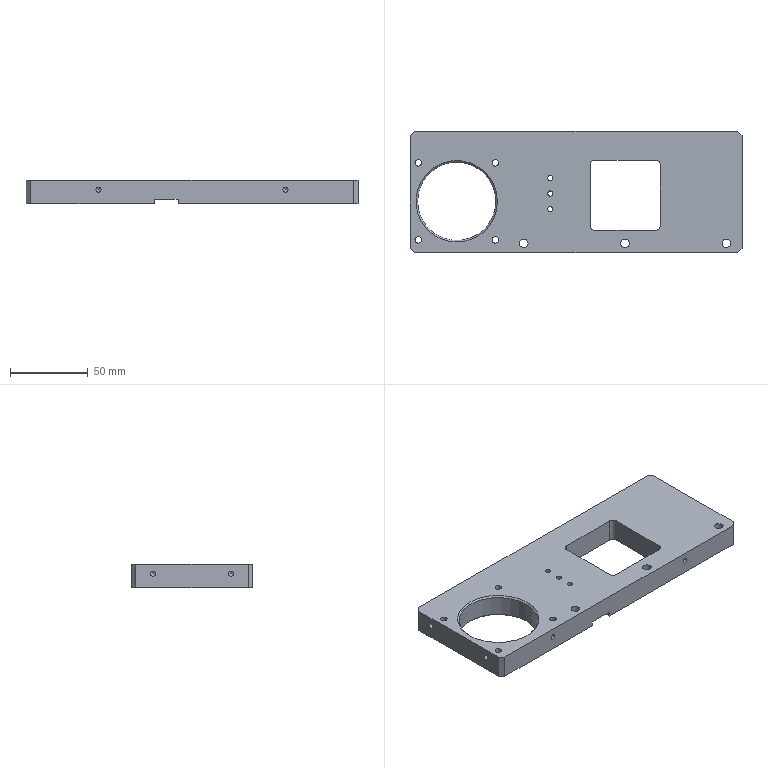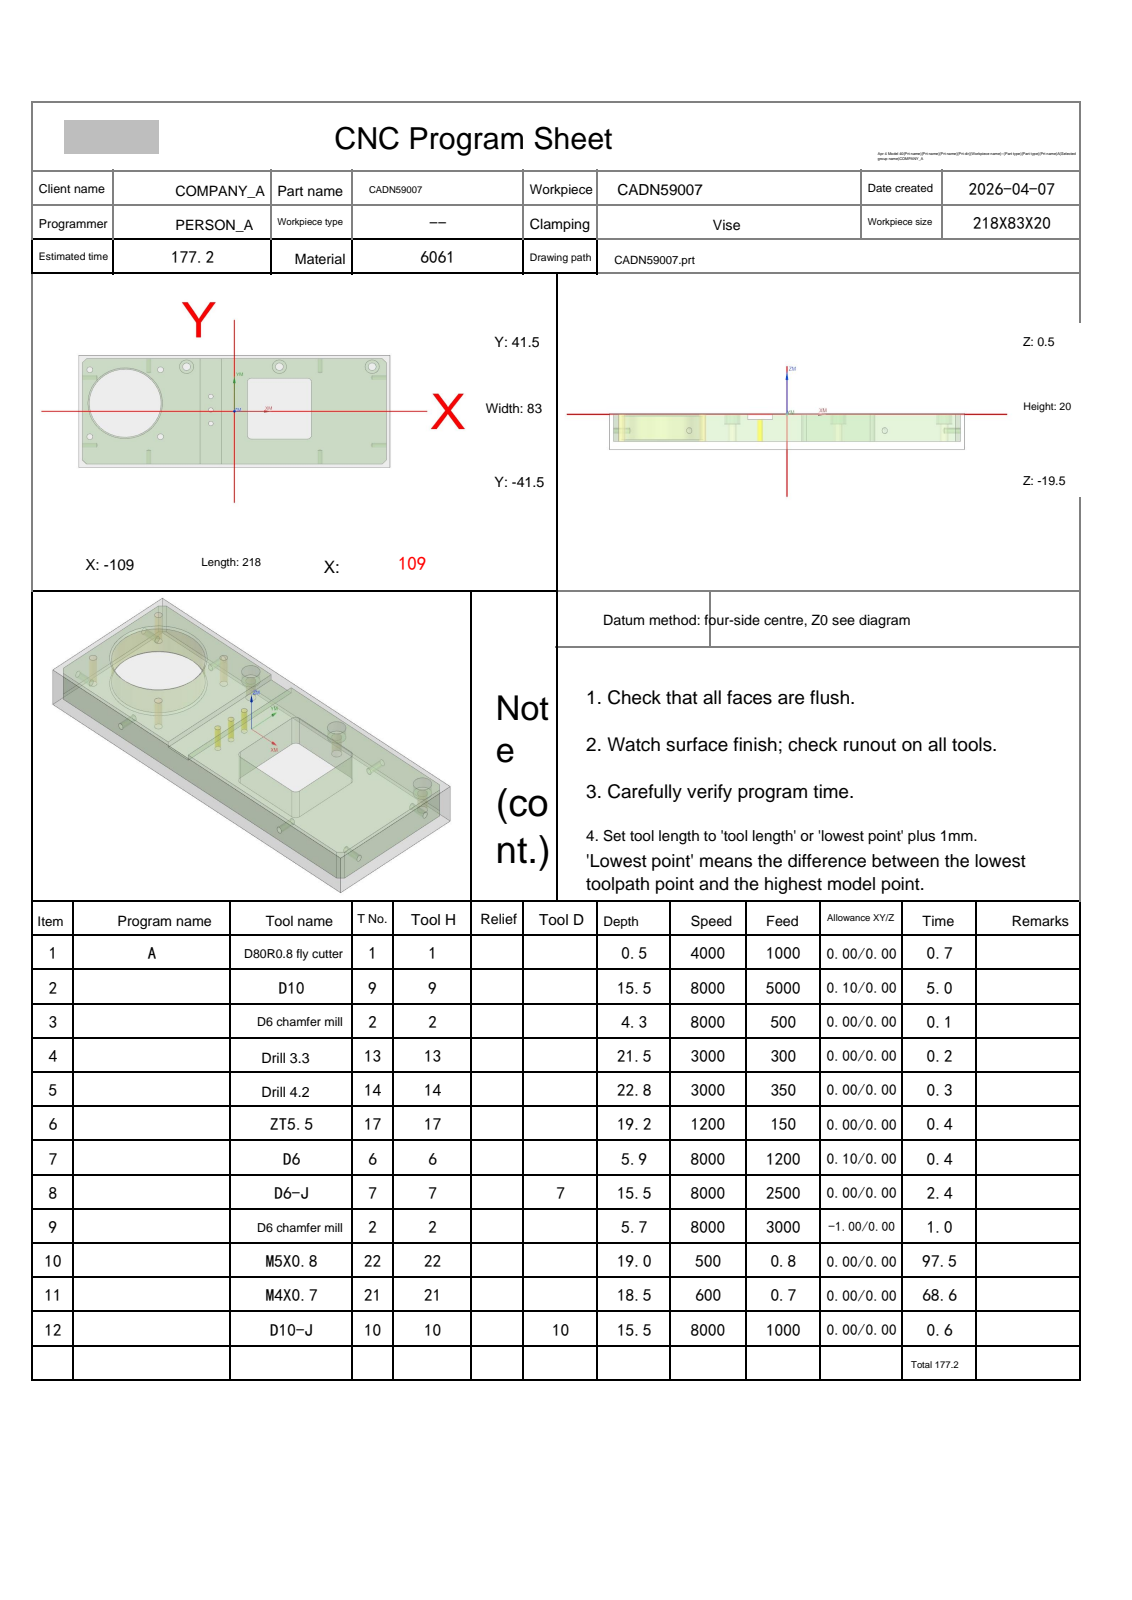NC program | NX | posted by the shop | part box 213 x 78 x 15 mm
Lines 7121 to 7501 of 7501:
N9 T02 M06
(D6 chamfer mill  D=6. R=0. H=02 ce=0.00 di=0.00)
G00 G90 G54 X47.025 Y41.128 M03 S8000
G43 H02 Z20.
M08
Z2.099
G01 Z-1.5 F3000.
G03 X46.945 Y40.828 I.52 J-.3
X47.245 Y40.308 I.6 J0.0
G01 X47.275 Y40.3
X103.5
X103.754 Y40.275
X103.997 Y40.201
X104.222 Y40.081
X104.419 Y39.919
X107.419 Y36.919
X107.581 Y36.722
X107.701 Y36.497
X107.775 Y36.254
X107.8 Y36.
Y-36.
X107.775 Y-36.254
X107.701 Y-36.497
X107.581 Y-36.722
X107.419 Y-36.919
X104.419 Y-39.919
X104.222 Y-40.081
X103.997 Y-40.201
X103.754 Y-40.275
X103.5 Y-40.3
X-8.95
G02 X-10.25 Y-39. I0.0 J1.3
G01 Y39.
G02 X-8.95 Y40.3 I1.3 J0.0
G01 X47.275
X47.305 Y40.308
G03 X47.605 Y40.828 I-.3 J.52
X47.525 Y41.128 I-.6 J0.0
G01 Z2.099
G00 Z20.
X11.128 Y2.25
Z2.099
G01 Z-1.5
G03 X10.828 Y2.33 I-.3 J-.52
X10.308 Y2.03 I0.0 J-.6
G01 X10.3 Y2.
Y-17.5
G03 X12. Y-19.2 I1.7 J0.0
G01 X51.
G03 X52.7 Y-17.5 I0.0 J1.7
G01 Y21.5
G03 X51. Y23.2 I-1.7 J0.0
G01 X12.
G03 X10.3 Y21.5 I0.0 J-1.7
G01 Y2.
X10.308 Y1.97
G03 X10.828 Y1.67 I.52 J.3
X11.128 Y1.75 I0.0 J.6
G01 Z2.099
G00 Z20.
X-21.922 Y.25
Z2.099
G01 Z-1.5
G03 X-22.222 Y.33 I-.3 J-.52
X-22.742 Y.03 I0.0 J-.6
G01 X-22.75 Y0.0
Y-39.
G02 X-24.05 Y-40.3 I-1.3 J0.0
G01 X-103.5
X-103.754 Y-40.275
X-103.997 Y-40.201
X-104.222 Y-40.081
X-104.419 Y-39.919
X-107.419 Y-36.919
X-107.581 Y-36.722
X-107.701 Y-36.497
X-107.775 Y-36.254
X-107.8 Y-36.
Y36.
X-107.775 Y36.254
X-107.701 Y36.497
X-107.581 Y36.722
X-107.419 Y36.919
X-104.419 Y39.919
X-104.222 Y40.081
X-103.997 Y40.201
X-103.754 Y40.275
X-103.5 Y40.3
X-24.05
G02 X-22.75 Y39. I0.0 J-1.3
G01 Y0.0
X-22.742 Y-.03
G03 X-22.222 Y-.33 I.52 J.3
X-21.922 Y-.25 I0.0 J.6
G01 Z2.099
G00 Z20.
X-11.999 Y-41.045
Z1.755
G01 Z-4.5
G03 X-11.927 Y-40.775 I-.468 J.27
X-12.197 Y-40.307 I-.54 J0.0
G01 X-12.224 Y-40.3
X-20.776
X-20.803 Y-40.307
G03 X-21.073 Y-40.775 I.27 J-.468
X-21.001 Y-41.045 I.54 J0.0
G01 Z1.755
G00 Z20.
Y41.045
Z1.755
G01 Z-4.5
G03 X-21.073 Y40.775 I.468 J-.27
X-20.803 Y40.307 I.54 J0.0
G01 X-20.776 Y40.3
X-12.224
X-12.197 Y40.307
G03 X-11.927 Y40.775 I-.27 J.468
X-11.999 Y41.045 I-.54 J0.0
G01 Z1.755
G00 Z20.
G00 G90 X-16.5 Y11. M03 S8000
Z20.
G98 G81 X-16.5 Y11. Z-5.2 R0.0 F500.
Y1.
Y-9.
G80
G00 Z20.
G00 G90 X-101.341 Y31.443 M03 S8000
Z20.
Z-.5
G01 Z-1. F500.
X-101.449 Y32.249
G03 X-102.949 Y30.749 I0.0 J-1.5
X-101.249 Y29.049 I1.7 J0.0
X-99.549 Y30.749 I0.0 J1.7
X-101.249 Y32.449 I-1.7 J0.0
X-102.949 Y30.749 I0.0 J-1.7
X-101.449 Y29.249 I1.5 J0.0
G01 X-101.341 Y30.055
Z-.5
G00 Z20.
Y-18.055
Z-.5
G01 Z-1.
X-101.449 Y-17.249
G03 X-102.949 Y-18.749 I0.0 J-1.5
X-101.249 Y-20.449 I1.7 J0.0
X-99.549 Y-18.749 I0.0 J1.7
X-101.249 Y-17.049 I-1.7 J0.0
X-102.949 Y-18.749 I0.0 J-1.7
X-101.449 Y-20.249 I1.5 J0.0
G01 X-101.341 Y-19.443
Z-.5
G00 Z20.
X-51.844 Y-18.055
Z-.5
G01 Z-1.
X-51.951 Y-17.249
G03 X-53.451 Y-18.749 I0.0 J-1.5
X-51.751 Y-20.449 I1.7 J0.0
X-50.051 Y-18.749 I0.0 J1.7
X-51.751 Y-17.049 I-1.7 J0.0
X-53.451 Y-18.749 I0.0 J-1.7
X-51.951 Y-20.249 I1.5 J0.0
G01 X-51.844 Y-19.443
Z-.5
G00 Z20.
Y31.443
Z-.5
G01 Z-1.
X-51.951 Y32.249
G03 X-53.451 Y30.749 I0.0 J-1.5
X-51.751 Y29.049 I1.7 J0.0
X-50.051 Y30.749 I0.0 J1.7
X-51.751 Y32.449 I-1.7 J0.0
X-53.451 Y30.749 I0.0 J-1.7
X-51.951 Y29.249 I1.5 J0.0
G01 X-51.844 Y30.055
Z-.5
G00 Z20.
G00 G90 X-30.846 Y36.386 M03 S8000
Z20.
Z2.5
G01 X-30.855 Y36.394 Z2.495 F800.
X-31.211 Y36.644 Z2.337
X-31.489 Y36.804 Z2.22
X-31.883 Y36.988 Z2.062
X-32.293 Y37.13 Z1.904
X-32.716 Y37.231 Z1.746
X-33.146 Y37.288 Z1.588
X-33.58 Y37.302 Z1.43
X-34.014 Y37.272 Z1.272
X-34.442 Y37.199 Z1.114
X-34.86 Y37.082 Z.956
X-35.265 Y36.924 Z.797
X-35.652 Y36.727 Z.639
X-36.016 Y36.491 Z.481
X-36.355 Y36.219 Z.323
X-36.665 Y35.915 Z.165
X-36.943 Y35.581 Z.007
X-37.186 Y35.221 Z-.151
X-37.391 Y34.838 Z-.309
X-37.556 Y34.436 Z-.467
X-37.68 Y34.02 Z-.625
X-37.762 Y33.593 Z-.783
X-37.8 Y33.161 Z-.942
Y33. Z-1.
G03 X-33.5 Y28.7 I4.3 J0.0
X-29.2 Y33. I0.0 J4.3
X-33.5 Y37.3 I-4.3 J0.0
X-37.8 Y33. I0.0 J-4.3
X-37.771 Y32.501 I4.3 J0.0
G01 Z1.5
G00 Z20.
X34.154 Y36.386
Z2.5
G01 X34.145 Y36.394 Z2.495
X33.789 Y36.644 Z2.337
X33.511 Y36.804 Z2.22
X33.117 Y36.988 Z2.062
X32.707 Y37.13 Z1.904
X32.284 Y37.231 Z1.746
X31.854 Y37.288 Z1.588
X31.42 Y37.302 Z1.43
X30.986 Y37.272 Z1.272
X30.558 Y37.199 Z1.114
X30.14 Y37.082 Z.956
X29.735 Y36.924 Z.797
X29.349 Y36.727 Z.639
X28.984 Y36.491 Z.481
X28.645 Y36.219 Z.323
X28.335 Y35.915 Z.165
X28.057 Y35.581 Z.007
X27.814 Y35.221 Z-.151
X27.609 Y34.838 Z-.309
X27.444 Y34.436 Z-.467
X27.32 Y34.02 Z-.625
X27.238 Y33.593 Z-.783
X27.2 Y33.161 Z-.942
Y33. Z-1.
G03 X31.5 Y28.7 I4.3 J0.0
X35.8 Y33. I0.0 J4.3
X31.5 Y37.3 I-4.3 J0.0
X27.2 Y33. I0.0 J-4.3
X27.229 Y32.501 I4.3 J0.0
G01 Z1.5
G00 Z20.
X99.154 Y36.386
Z2.5
G01 X99.145 Y36.394 Z2.495
X98.789 Y36.644 Z2.337
X98.511 Y36.804 Z2.22
X98.117 Y36.988 Z2.062
X97.707 Y37.13 Z1.904
X97.284 Y37.231 Z1.746
X96.854 Y37.288 Z1.588
X96.42 Y37.302 Z1.43
X95.986 Y37.272 Z1.272
X95.558 Y37.199 Z1.114
X95.14 Y37.082 Z.956
X94.735 Y36.924 Z.797
X94.349 Y36.727 Z.639
X93.984 Y36.491 Z.481
X93.645 Y36.219 Z.323
X93.335 Y35.915 Z.165
X93.057 Y35.581 Z.007
X92.814 Y35.221 Z-.151
X92.609 Y34.838 Z-.309
X92.444 Y34.436 Z-.467
X92.32 Y34.02 Z-.625
X92.238 Y33.593 Z-.783
X92.2 Y33.161 Z-.942
Y33. Z-1.
G03 X96.5 Y28.7 I4.3 J0.0
X100.8 Y33. I0.0 J4.3
X96.5 Y37.3 I-4.3 J0.0
X92.2 Y33. I0.0 J-4.3
X92.229 Y32.501 I4.3 J0.0
G01 Z1.5
G00 Z20.
G00 G90 X-55.85 Y3. M03 S8000
Z20.
Z-1.5
G01 Z-2. F800.
G03 X-52.85 Y6. I0.0 J3.
X-76.5 Y29.65 I-23.65 J0.0
X-100.15 Y6. I0.0 J-23.65
X-76.5 Y-17.65 I23.65 J0.0
X-52.85 Y6. I0.0 J23.65
X-55.85 Y9. I-3. J0.0
G01 Z-1.5
G00 Z20.
G00 G90 X-55.35 Y3. M03 S8000
Z20.
Z-1.5
G01 Z-2. F800.
G03 X-52.35 Y6. I0.0 J3.
X-76.5 Y30.15 I-24.15 J0.0
X-100.65 Y6. I0.0 J-24.15
X-76.5 Y-18.15 I24.15 J0.0
X-52.35 Y6. I0.0 J24.15
X-55.35 Y9. I-3. J0.0
G01 Z-1.5
G00 Z20.
G91 G28 Z0.0
M05
M09
G91 G28 Z0.0
M01
N10 T22 M06
(M5X0.8 D=4.2 DR_a=180 H=22)
G00 G90 G54 X-51.751 Y30.749 M03 S500
G43 H22 Z20.
M08
G95
G98 G84 X-51.751 Y30.749 Z-18.5 R1. F.8 Q3.
X-101.249
Y-18.749
X-51.751
G80
G94
G00 Z20.
G91 G28 Z0.0
M05
M09
G91 G28 Z0.0
M01
N11 T21 M06
(M4X0.7 D=3.3 DR_a=180 H=21)
G00 G90 G54 X-16.5 Y11. M03 S600
G43 H21 Z20.
M08
G95
G98 G84 X-16.5 Y11. Z-18. R-2. F.7 Q4.
Y1.
Y-9.
G80
G94
G00 Z20.
G91 G28 Z0.0
M05
M09
G91 G28 Z0.0
M01
N12 T10 M06
(D10-J  D=10. R=0. H=10 ce=0.00 di=0.00)
G00 G90 G54 X104.513 Y-45.116 M03 S8000
G43 H10 Z20.
M08
Z-14.5
G01 Z-15. F1000.
G41 D10
X104.497 Y-44.917
G03 X103.5 Y-44. I-.997 J-.083
G01 X-103.5
G02 X-107.036 Y-42.536 I0.0 J5.
G01 X-110.036 Y-39.536
G02 X-111.5 Y-36. I3.536 J3.536
G01 Y36.
G02 X-110.036 Y39.536 I5. J0.0
G01 X-107.036 Y42.536
G02 X-103.5 Y44. I3.536 J-3.536
G01 X103.5
G02 X107.036 Y42.536 I0.0 J-5.
G01 X110.036 Y39.536
G02 X111.5 Y36. I-3.536 J-3.536
G01 Y-36.
G02 X110.036 Y-39.536 I-5. J0.0
G01 X107.036 Y-42.536
G02 X103.5 Y-44. I-3.536 J3.536
G01 X103.
G03 X102. Y-45. I0.0 J-1.
G01 G40 Y-45.2
Z-14.5
G00 Z20.
M05
M09
G91 G28 Z0.0
G91 G28 Y0.0
M30
%